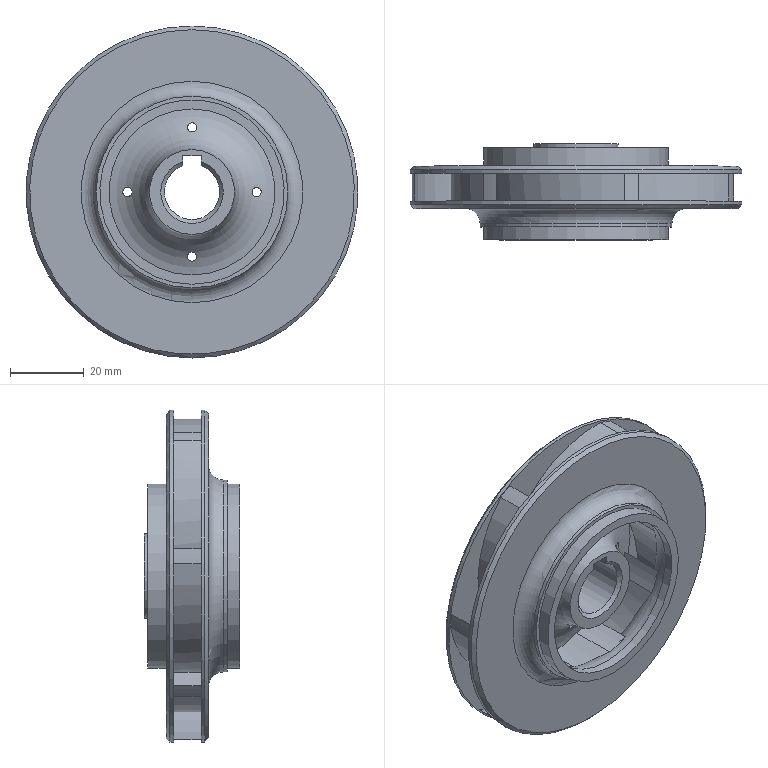Part | NX | features DATUM_CSYS 5, SKETCH 4, EXTRUDE 3, CHAMFER 1, REPLACE_FACE 1, SWP104 1, UNITE 1 | 1 solid | 61 faces | box 90 x 26 x 90 mm | volume 37267 mm3 | cylinder 41 | plane 13 | torus 4 | cone 3 | commonest cylinder face diameters 46 x7 70 x7 72 x7 89 x7 2.5 x4 45 x2